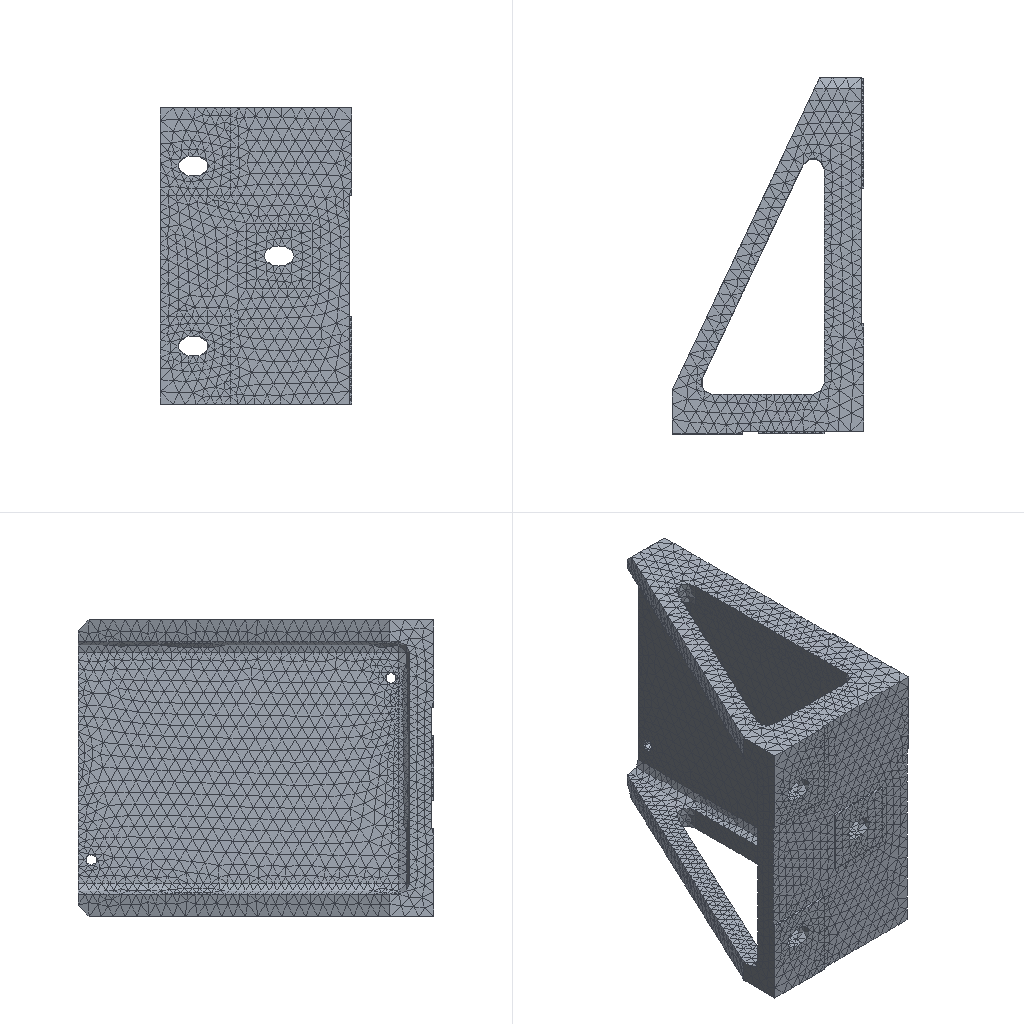Simulation study | nx simcenter
Set-up summary:
category,name,step,type,value,unit,region
solver,nx_nastran (Simcenter)
units,not stated in the deck,,not stated
analysis,deck,,static,static
analysis,solution,,SOL,101
load_step,SUBCASE 1,1,SUBCASE,SPC=1 LOAD=2
load_step,requested,,,1
mesh,nodes,,,37618
mesh,elements,,,21095
element_type,CTETRA,,solid,21095
load,nodal force total,,FX,3499999.909,model units
load,nodal force total,,FY,0.0,model units
load,nodal force total,,FZ,0.0,model units
load,load commands in deck,,count,637
bc,support commands in deck,,count,900
analysis,NX solution 0,,Structural,Linear Statics - Single Constraint
check,setup vs results,,match,every grid point's frame and coordinates and every element id; grid points of CTETRA elements
Nastran input file, long lists of numbers shortened:
$*$$$$$$$$$$$$$$$$$$$$$$$$$$$$$$$$$$$$$$$$$$$$$$$$$$$$$$$$$$$$$$$$$
$*
$*                    NX v10.0.0.24 TRANSLATOR
$*                    FOR NX NASTRAN VERSION 10.0
$ (33 more lines like these left out)
ASSIGN OUTPUT2='154_sim1-solution_1.op2' UNIT=12
$*
$*$$$$$$$$$$$$$$$$$$$$$$$$$$$$$$$$$$$
$*
$* EXECUTIVE CONTROL
$*
$*$$$$$$$$$$$$$$$$$$$$$$$$$$$$$$$$$$$
$*
ID,NASTRAN,154_sim1-solution_1
SOL 101
CEND
$*
$*$$$$$$$$$$$$$$$$$$$$$$$$$$$$$$$$$$$
$*
$* CASE CONTROL
$*
$*$$$$$$$$$$$$$$$$$$$$$$$$$$$$$$$$$$$
$*
TITLE = Solution 1
ECHO = NONE
SPC = 1
OUTPUT
BCRESULTS(TRACTION,FORCE,PLOT) = ALL
DISPLACEMENT(PLOT) = ALL
ESE(PLOT) = ALL
FORCE(PLOT,CORNER) = ALL
OLOAD(PLOT) = ALL
SPCFORCES(PLOT) = ALL
STRAIN(PLOT,FIBER,CORNER) = ALL
STRESS(PLOT,CORNER) = ALL
$*  NX Step: Subcase - Static Loads 1
SUBCASE 1
LABEL = Subcase - Static Loads 1
LOAD = 2
$*
$*$$$$$$$$$$$$$$$$$$$$$$$$$$$$$$$$$$$
$*
$* BULK DATA
$*
$*$$$$$$$$$$$$$$$$$$$$$$$$$$$$$$$$$$$
$*
BEGIN BULK
$*
$* PARAM CARDS
$*
PARAM      K6ROT100.0000
PARAM     OIBULK     YES
PARAM    OMACHPR     YES
PARAM       POST      -2
PARAM    POSTEXT     YES
PARAM    UNITSYS   MN-MM
$*
$* GRID CARDS
$*
GRID*              37492               0-8.700000000E+011.0000000000E+01+
*       2.5000000000E+01               0
GRID*              37493               0-8.700000000E+011.0000000000E+01+
*       -1.500000000E+01               0
$ (75232 more lines like these left out)
$*
$* ELEMENT CARDS
$*
$*  NX Mesh Collector: Solid(1)
$*  NX Mesh: 3d_mesh(1)
CTETRA         1       1   36814   34701   37588   36813   34730    1403+
+          26974   36819   34729   26973
CTETRA         2       1   31564   31574       1       2   32527    1404+
+           1405    1406    1407    1408
$ (42186 more lines like these left out)
$*
$* PROPERTY CARDS
$*
$*  NX Property: PSOLID1
PSOLID         1       1       0                           SMECH
$*
$* MATERIAL CARDS
$*
$*  NX Material: ZL114A
MAT1           17.1000+7        0.3300002.6850-62.5000-5
$*
$* LOAD AND CONSTRAINT CARDS
$*
$*  NX Load and Constraint: Fixed(1)
SPC            1   19892  123456  0.0000
SPC            1   19893  123456  0.0000
SPC            1   19894  123456  0.0000
SPC            1   19895  123456  0.0000
$ (896 more lines like these left out)
$*  NX Load and Constraint: Force(1)
FORCE          2   29944       0 4004.621.000000  0.0000  0.0000
FORCE          2   29945       0 4023.331.000000  0.0000  0.0000
FORCE          2   29946       0 3978.961.000000  0.0000  0.0000
FORCE          2   29947       0 4214.291.000000  0.0000  0.0000
$ (633 more lines like these left out)
ENDDATA 0cd7dc61
Results summary:
result,analysis,,,static
result,last_loadstep,,,1
result,primary field,,,displacements
result,reaction total,,FX,-3500001.5,model units
result,reaction total,,FY,0.4219,model units
result,reaction total,,FZ,0.1138,model units
result,NX solution 0,,loadcases,1,mm